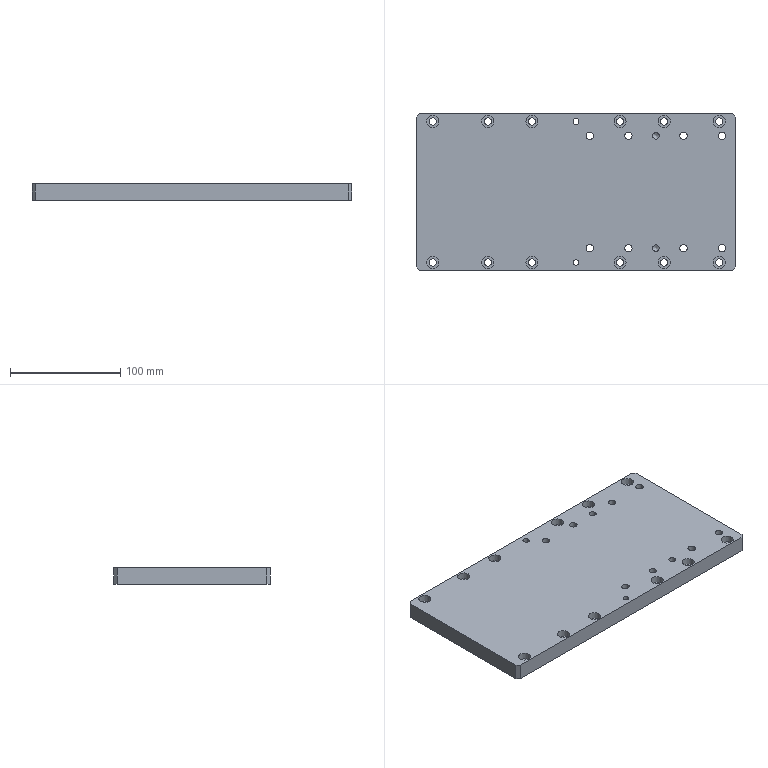CAM job | NX | 3-axis milling, drilling | part box 290 x 142 x 15 mm | stock box 295 x 147 x 20 mm
Tools:
number,name,description,diameter,corner_radius,flute_length,length,flutes
3,D3,平底铣刀-粗,3.0,0.0,20.0,75.0,2
6,D6,平底铣刀-粗,6.0,0.0,25.0,75.0,2
9,D10,平底铣刀-粗,10.0,0.0,35.0,75.0,2
11,D3-J,平底铣刀-精,3.0,0.0,50.0,75.0,2
7,D6-J,平底铣刀-精,6.0,0.0,25.0,75.0,2
10,D10-J,平底铣刀-精,10.0,0.0,35.0,75.0,2
1,D80R0.8_FACEMILL,圆鼻刀-粗,80.0,0.8,50.0,75.0,2
1,D80R0.8_FACEMILL-J,圆鼻刀-精,80.0,0.8,50.0,75.0,2
2,D6_CHAMFERMILL,倒角刀,6.0,0.0,3.0,25.0,2
24,M8X1.25,丝锥,6.8,0.0,35.0,50.0,2
23,D5_REAMER,Drilling Tool,5.0,0.0,75.0,100.0,6
18,ZT5.8,钻头,5.8,0.0,35.0,50.0,2
19,ZT6.6,钻头,6.6,0.0,35.0,50.0,2
16,ZT6.8,钻头,6.8,0.0,35.0,50.0,2
17,ZT4.9,Drilling Tool,4.9,0.0,35.0,50.0,2
Operations:
program,operation,operation_type,tool,method,geometry_group,spindle_rpm,surface_speed,feed_per_tooth,feed_cut,feed_plunge,cut_length_mm,path_length_mm,cut_time_min,machine_time_min
B,FLOOR_WALL_FACEMILL_ROUGH_COPY,VolumeBased25DMillingOperation,D80R0.8_FACEMILL,Z_LEVEL_ROUGH-DEPTHK-STEPG,W-B,2800.0,703.696,0.5357,3000.0,100.0,10911.308,14339.132,3.637,3.98
B,FLOOR_WALL_FACEMILL_FINISH_COPY,VolumeBased25DMillingOperation,D80R0.8_FACEMILL-J,SIDE_FINISH-DEPTHK-STEPG,W-B,4000.0,1005.28,0.125,1000.0,100.0,1211.584,1247.584,1.212,1.215
B,DRILL_CHAMFER_DJ10_1,Operation,D6_CHAMFERMILL,METHOD,W-B,8000.0,150.796,0.0625,1000.0,0.0,5.8,51.6,0.0058,0.0104
B,MILL_CHAMFER_5,PlanarMilling,D6_CHAMFERMILL,METHOD,W-B,8000.0,150.796,0.075,1200.0,100.0,245.352,1397.611,0.2045,0.3197
B,MILL_CHAMFER_6,PlanarMilling,D6_CHAMFERMILL,METHOD,W-B,8000.0,150.796,0.0375,600.0,100.0,250.195,931.826,0.417,0.4852
B,C0.3_CLOSED_CONTOUR_CHAMFER6X45L_COPY,PlanarMilling,D6_CHAMFERMILL,CLIMB_CHAMFER-DEPTH0-STEPG,W-B,7000.0,131.0,0.1071,1500.0,100.0,901.042,1170.529,0.6007,0.6276
A,TOP_FACE,FaceMilling,D80R0.8_FACEMILL,SIDE_FINISH-DEPTHK-STEPG,W-A,4000.0,1005.31,0.125,1000.0,100.0,1627.2,1663.2,1.627,1.631
A,PROFILE_ROUGH_2,VolumeBased25DMillingOperation,D10,METHOD,W-A,8000.0,251.327,0.3125,5000.0,80.0,18670.818,18724.818,3.734,3.74
A,SPOT-DEPTH0.8,Operation,D6_CHAMFERMILL,NONE,W-A,8000.0,150.796,0.0312,500.0,90.0,43.2,1037.02,0.0864,0.1858
A,THROUGH_HOLE-FINISH6.0_PILOT,Operation,ZT4.9,NONE,W-A,2500.0,38.484,0.05,250.0,90.0,40.829,250.162,0.1633,0.1842
A,THROUGH_HOLE-FINISH6.0_PILOT14.8,Operation,ZT5.8,NONE,W-A,2500.0,45.553,0.03,150.0,90.0,19.405,181.815,0.1294,0.1456
A,COUNTERBORE-DRILL_SEG0,Operation,ZT6.6,NONE,W-A,1200.0,24.881,0.0625,150.0,90.0,239.794,1178.695,1.599,1.692
A,THROUGH_HOLE-M8_TAP_DRILL,Operation,ZT6.8,NONE,W-A,1800.0,38.453,0.0972,350.0,90.0,200.343,789.769,0.5724,0.6314
A,MILL_HOLE_ROUGH_D6_1,CylinderMilling,D6,NONE,W-A,8000.0,150.796,0.075,1200.0,100.0,2769.995,3968.795,2.308,2.428
A,MILL_HOLE_FINISH_D6_1,CylinderMilling,D6-J,FINISH_STEP_DEPTH_OFF,W-A,8000.0,150.796,0.0312,500.0,100.0,535.384,1740.184,1.071,1.191
A,THROUGH_SLOT_ROUGH_1,VolumeBased25DMillingOperation,D3,METHOD,W-A,6000.0,56.549,0.0417,500.0,100.0,862.305,916.305,1.725,1.73
A,MILL_HOLE_ROUGH_D4_2,CylinderMilling,D3,NONE,W-A,8000.0,100.531,0.0375,600.0,100.0,479.781,674.781,0.7996,0.8191
A,SELECTED_BODY_ONLY,SurfaceContour,D6_CHAMFERMILL,METHOD,W-A,8000.0,150.796,0.1875,3000.0,100.0,892.959,1101.938,0.2977,0.3186
A,MILL_CHAMFER_1,PlanarMilling,D6_CHAMFERMILL,METHOD,W-A,8000.0,150.796,0.0312,500.0,100.0,18.482,59.481,0.037,0.0411
A,MILL_CHAMFER_2,PlanarMilling,D6_CHAMFERMILL,METHOD,W-A,8000.0,150.796,0.0312,500.0,100.0,41.927,223.633,0.0839,0.102
A,MILL_CHAMFER_3,PlanarMilling,D6_CHAMFERMILL,METHOD,W-A,8000.0,150.796,0.0375,600.0,100.0,195.21,867.703,0.3253,0.3926
A,MILL_CHAMFER_4,PlanarMilling,D6_CHAMFERMILL,NONE,W-A,8000.0,150.796,0.05,800.0,100.0,520.711,1598.506,0.6509,0.7587
A,REAM_HOLE,Operation,D5_REAMER,METHOD,W-A,500.0,7.854,0.0167,50.0,0.0,17.0,74.0,0.34,0.3457
A,MILL_HOLE_FINISH_D4-J_2,CylinderMilling,D3-J,FINISH_STEP_DEPTH_OFF,W-A,8000.0,100.531,0.0125,200.0,100.0,171.417,366.417,0.8571,0.8766
A,SLOT_FINISH_1,VolumeBased25DMillingOperation,D3-J,METHOD,W-A,6000.0,56.549,0.0167,200.0,100.0,31.798,122.599,0.159,0.1681
A,THROUGH_HOLE-TAP_M8,Operation,M8X1.25,METHOD,W-A,500.0,10.681,0.0013,1.25,90.0,160.0,709.082,128.0,128.055
A,PROFILE_SEMIFINISH_2,VolumeBased25DMillingOperation,D10-J,METHOD,W-A,8000.0,251.327,0.0625,1000.0,100.0,893.345,963.345,0.8933,0.9003